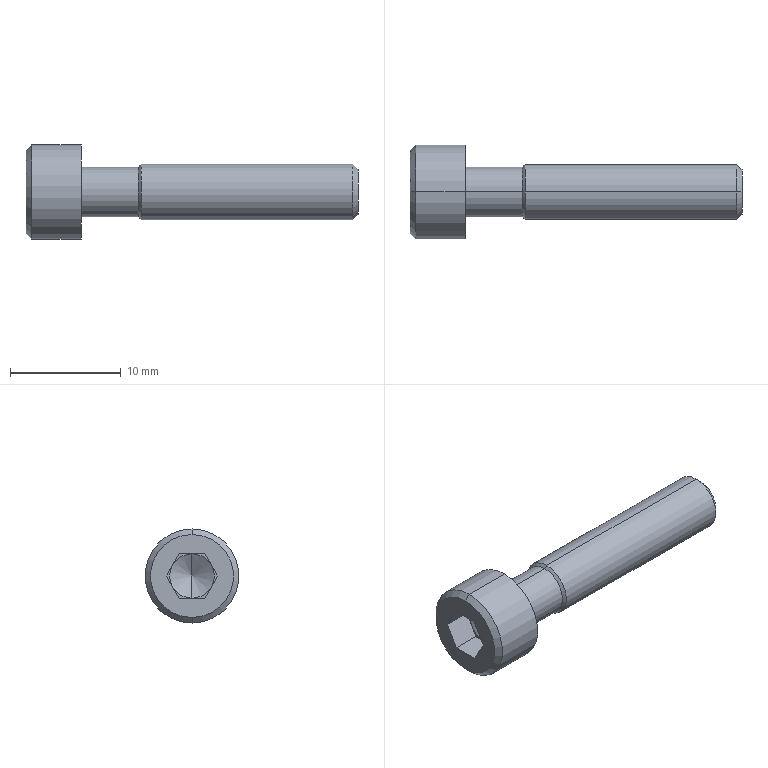Part | STEP file | 0232_Z_SCBS5-25_1 | 1 solid | 29 faces | box 30 x 8.5 x 8.5 mm | volume 710.772 mm3 | plane 15 | cone 8 | cylinder 6 | commonest cylinder face diameters 4.509 x2 5 x2 8.5 x2